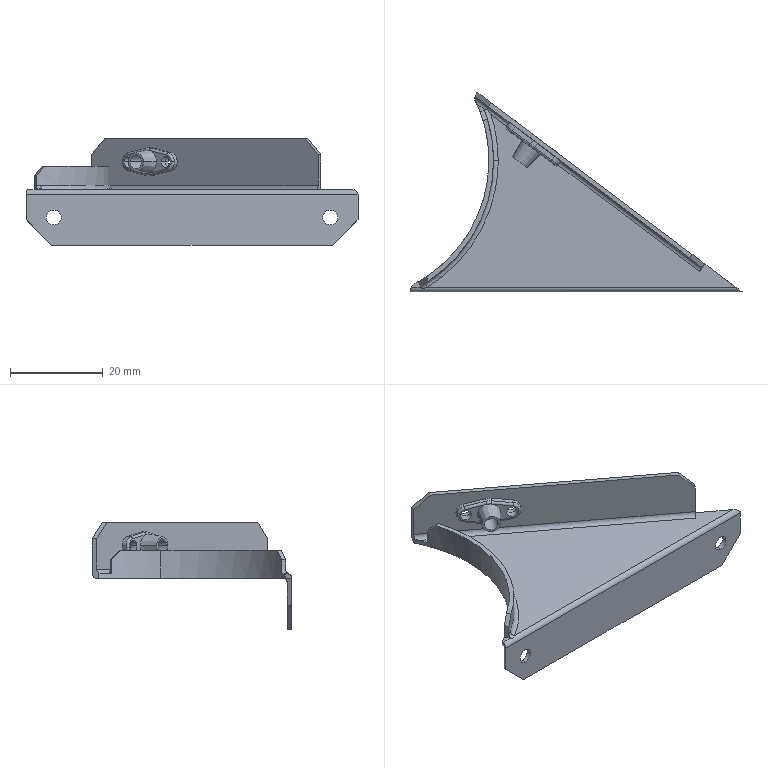Part | SolidWorks | features BaseBody 3 | 3 solids | 80 faces | box 71.5 x 43.03 x 23 mm | volume 2990 mm3 | cylinder 35 | plane 33 | spline 10 | cone 2 | commonest cylinder face diameters 2.4 x8 3 x6 2 x5 1 x4 3.2 x4 4 x3